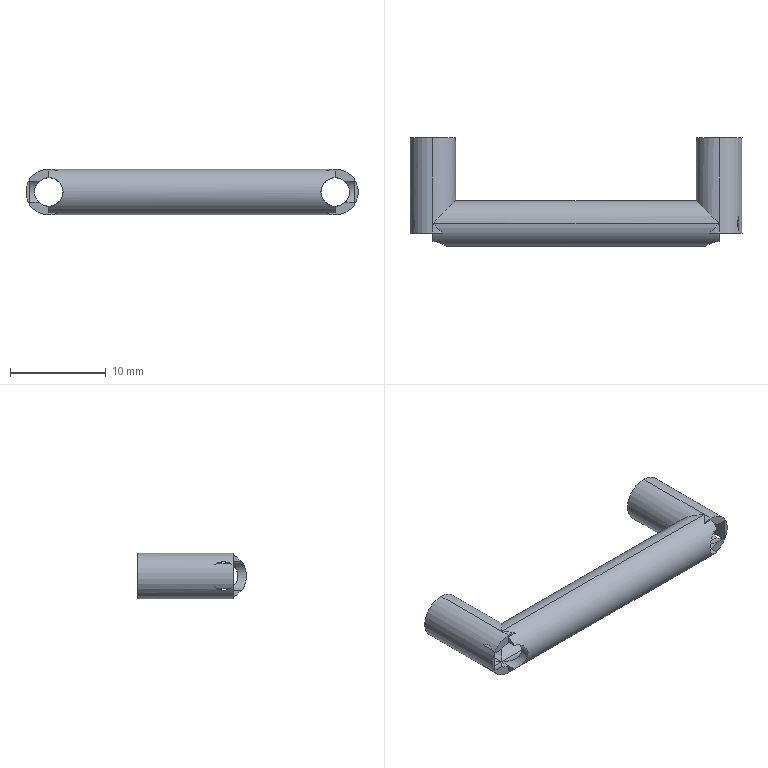Part | SolidWorks | features BaseBody 1 | 1 solid | 38 faces | box 34.8 x 11.4 x 4.8 mm | volume 496.257 mm3 | cylinder 28 | plane 10 | commonest cylinder face diameters 3 x18 4.8 x10